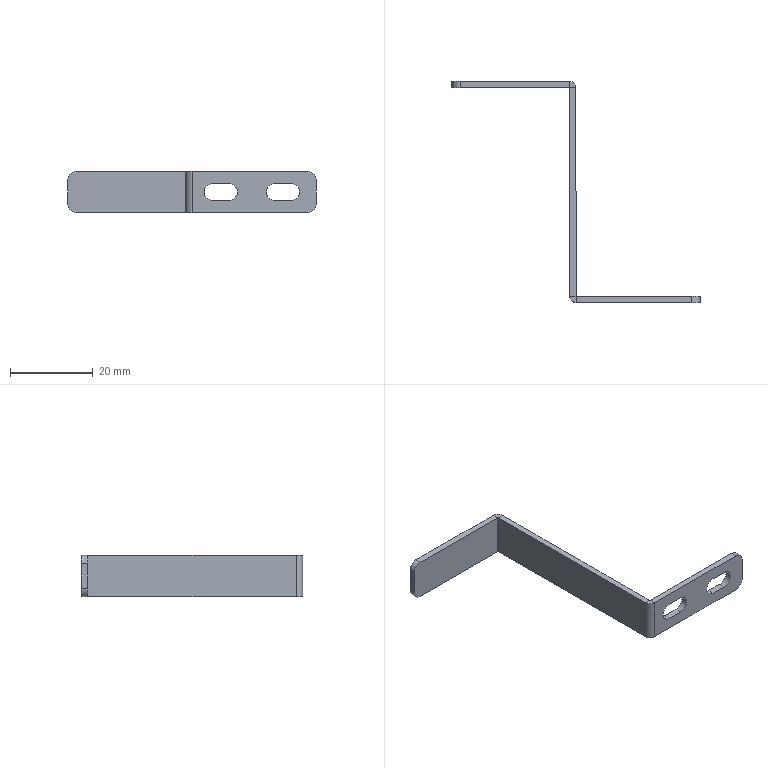Part | SolidWorks | features BreakCorner 1, FlatPattern 1, HoleWzd 1, SMBaseFlange 1, SheetMetal 1 | 1 solid | 34 faces | box 60 x 53.5 x 10 mm | volume 1574 mm3 | plane 22 | cylinder 12 | commonest cylinder face diameters 4 x4 4.2 x4 0.2 x2 3.2 x2
STEP:
#1=CARTESIAN_POINT('',(30.,-1.6,5.));
#2=VERTEX_POINT('',#1);
#3=CARTESIAN_POINT('',(28.5,-1.6,5.));
#4=VERTEX_POINT('',#3);
#5=CARTESIAN_POINT('',(30.,-1.6,5.));
#6=DIRECTION('',(-1.,0.,0.));
#7=VECTOR('',#6,1000.);
#8=LINE('',#5,#7);
#9=EDGE_CURVE('',#2,#4,#8,.T.);
#10=ORIENTED_EDGE('',*,*,#9,.F.);
#11=CARTESIAN_POINT('',(28.4,0.,5.));
#12=VERTEX_POINT('',#11);
#13=CARTESIAN_POINT('',(28.4,-1.6,5.));
#14=DIRECTION('',(0.,0.,-1.));
#15=DIRECTION('',(1.,0.,0.));
#16=AXIS2_PLACEMENT_3D('',#13,#14,#15);
#17=CIRCLE('',#16,1.6);
#18=EDGE_CURVE('',#12,#2,#17,.T.);
#19=ORIENTED_EDGE('',*,*,#18,.F.);
#20=CARTESIAN_POINT('',(28.4,-1.5,5.));
#21=VERTEX_POINT('',#20);
#22=CARTESIAN_POINT('',(28.4,-1.5,5.));
#23=DIRECTION('',(0.,1.,0.));
#24=VECTOR('',#23,1000.);
#25=LINE('',#22,#24);
#26=EDGE_CURVE('',#21,#12,#25,.T.);
#27=ORIENTED_EDGE('',*,*,#26,.F.);
#28=CARTESIAN_POINT('',(28.4,-1.6,5.));
#29=DIRECTION('',(0.,0.,-1.));
#30=DIRECTION('',(1.,0.,0.));
#31=AXIS2_PLACEMENT_3D('',#28,#29,#30);
#32=CIRCLE('',#31,0.1);
#33=EDGE_CURVE('',#21,#4,#32,.T.);
#34=ORIENTED_EDGE('',*,*,#33,.T.);
#35=EDGE_LOOP('',(#10,#19,#27,#34));
#36=FACE_OUTER_BOUND('',#35,.T.);
#37=CARTESIAN_POINT('',(30.,-1.6,5.));
#38=DIRECTION('',(0.,0.,1.));
#39=DIRECTION('',(1.,0.,0.));
#40=AXIS2_PLACEMENT_3D('',#37,#38,#39);
#41=PLANE('',#40);
#42=ADVANCED_FACE('',(#36),#41,.T.);
#43=CARTESIAN_POINT('',(30.,-51.9,5.));
#44=VERTEX_POINT('',#43);
#45=CARTESIAN_POINT('',(30.,0.,5.));
#46=DIRECTION('',(0.,-1.,0.));
#47=VECTOR('',#46,1000.);
#48=LINE('',#45,#47);
#49=EDGE_CURVE('',#2,#44,#48,.T.);
#50=ORIENTED_EDGE('',*,*,#49,.F.);
#51=ORIENTED_EDGE('',*,*,#9,.T.);
#52=CARTESIAN_POINT('',(28.5,-51.9,5.));
#53=VERTEX_POINT('',#52);
#54=CARTESIAN_POINT('',(28.5,0.,5.));
#55=DIRECTION('',(0.,-1.,0.));
#56=VECTOR('',#55,1000.);
#57=LINE('',#54,#56);
#58=EDGE_CURVE('',#4,#53,#57,.T.);
#59=ORIENTED_EDGE('',*,*,#58,.T.);
#60=CARTESIAN_POINT('',(28.5,-51.9,5.));
#61=DIRECTION('',(1.,0.,0.));
#62=VECTOR('',#61,1000.);
#63=LINE('',#60,#62);
#64=EDGE_CURVE('',#53,#44,#63,.T.);
#65=ORIENTED_EDGE('',*,*,#64,.T.);
#66=EDGE_LOOP('',(#50,#51,#59,#65));
#67=FACE_OUTER_BOUND('',#66,.T.);
#68=CARTESIAN_POINT('',(28.4,-1.5,5.));
#69=DIRECTION('',(0.,0.,1.));
#70=DIRECTION('',(1.,0.,0.));
#71=AXIS2_PLACEMENT_3D('',#68,#69,#70);
#72=PLANE('',#71);
#73=ADVANCED_FACE('',(#67),#72,.T.);
#74=CARTESIAN_POINT('',(28.4,0.,-5.));
#75=VERTEX_POINT('',#74);
#76=CARTESIAN_POINT('',(28.4,-1.5,-5.));
#77=VERTEX_POINT('',#76);
#78=CARTESIAN_POINT('',(28.4,0.,-5.));
#79=DIRECTION('',(0.,-1.,0.));
#80=VECTOR('',#79,1000.);
#81=LINE('',#78,#80);
#82=EDGE_CURVE('',#75,#77,#81,.T.);
#83=ORIENTED_EDGE('',*,*,#82,.F.);
#84=CARTESIAN_POINT('',(30.,-1.6,-5.));
#85=VERTEX_POINT('',#84);
#86=CARTESIAN_POINT('',(28.4,-1.6,-5.));
#87=DIRECTION('',(0.,0.,-1.));
#88=DIRECTION('',(1.,0.,0.));
#89=AXIS2_PLACEMENT_3D('',#86,#87,#88);
#90=CIRCLE('',#89,1.6);
#91=EDGE_CURVE('',#75,#85,#90,.T.);
#92=ORIENTED_EDGE('',*,*,#91,.T.);
#93=CARTESIAN_POINT('',(28.5,-1.6,-5.));
#94=VERTEX_POINT('',#93);
#95=CARTESIAN_POINT('',(28.5,-1.6,-5.));
#96=DIRECTION('',(1.,0.,0.));
#97=VECTOR('',#96,1000.);
#98=LINE('',#95,#97);
#99=EDGE_CURVE('',#94,#85,#98,.T.);
#100=ORIENTED_EDGE('',*,*,#99,.F.);
#101=CARTESIAN_POINT('',(28.4,-1.6,-5.));
#102=DIRECTION('',(0.,0.,-1.));
#103=DIRECTION('',(1.,0.,0.));
#104=AXIS2_PLACEMENT_3D('',#101,#102,#103);
#105=CIRCLE('',#104,0.1);
#106=EDGE_CURVE('',#77,#94,#105,.T.);
#107=ORIENTED_EDGE('',*,*,#106,.F.);
#108=EDGE_LOOP('',(#83,#92,#100,#107));
#109=FACE_OUTER_BOUND('',#108,.T.);
#110=CARTESIAN_POINT('',(28.4,0.,-5.));
#111=DIRECTION('',(0.,0.,-1.));
#112=DIRECTION('',(-1.,0.,0.));
#113=AXIS2_PLACEMENT_3D('',#110,#111,#112);
#114=PLANE('',#113);
#115=ADVANCED_FACE('',(#109),#114,.T.);
#116=CARTESIAN_POINT('',(2.,-1.5,-5.));
#117=VERTEX_POINT('',#116);
#118=CARTESIAN_POINT('',(0.,-1.5,-5.));
#119=DIRECTION('',(1.,0.,0.));
#120=VECTOR('',#119,1000.);
#121=LINE('',#118,#120);
#122=EDGE_CURVE('',#117,#77,#121,.T.);
#123=ORIENTED_EDGE('',*,*,#122,.F.);
#124=CARTESIAN_POINT('',(2.,0.,-5.));
#125=VERTEX_POINT('',#124);
#126=CARTESIAN_POINT('',(2.,-1.6,-5.));
#127=DIRECTION('',(0.,1.,0.));
#128=VECTOR('',#127,1000.);
#129=LINE('',#126,#128);
#130=EDGE_CURVE('',#117,#125,#129,.T.);
#131=ORIENTED_EDGE('',*,*,#130,.T.);
#132=CARTESIAN_POINT('',(0.,0.,-5.));
#133=DIRECTION('',(1.,0.,0.));
#134=VECTOR('',#133,1000.);
#135=LINE('',#132,#134);
#136=EDGE_CURVE('',#125,#75,#135,.T.);
#137=ORIENTED_EDGE('',*,*,#136,.T.);
#138=ORIENTED_EDGE('',*,*,#82,.T.);
#139=EDGE_LOOP('',(#123,#131,#137,#138));
#140=FACE_OUTER_BOUND('',#139,.T.);
#141=CARTESIAN_POINT('',(28.5,-1.6,-5.));
#142=DIRECTION('',(0.,0.,-1.));
#143=DIRECTION('',(-1.,0.,0.));
#144=AXIS2_PLACEMENT_3D('',#141,#142,#143);
#145=PLANE('',#144);
#146=ADVANCED_FACE('',(#140),#145,.T.);
#147=CARTESIAN_POINT('',(30.1,-52.,5.));
#148=VERTEX_POINT('',#147);
#149=CARTESIAN_POINT('',(30.1,-53.5,5.));
#150=VERTEX_POINT('',#149);
#151=CARTESIAN_POINT('',(30.1,-52.,5.));
#152=DIRECTION('',(0.,-1.,0.));
#153=VECTOR('',#152,1000.);
#154=LINE('',#151,#153);
#155=EDGE_CURVE('',#148,#150,#154,.T.);
#156=ORIENTED_EDGE('',*,*,#155,.F.);
#157=CARTESIAN_POINT('',(30.1,-51.9,5.));
#158=DIRECTION('',(0.,0.,1.));
#159=DIRECTION('',(-1.,0.,0.));
#160=AXIS2_PLACEMENT_3D('',#157,#158,#159);
#161=CIRCLE('',#160,0.1);
#162=EDGE_CURVE('',#44,#148,#161,.T.);
#163=ORIENTED_EDGE('',*,*,#162,.F.);
#164=ORIENTED_EDGE('',*,*,#64,.F.);
#165=CARTESIAN_POINT('',(30.1,-51.9,5.));
#166=DIRECTION('',(0.,0.,1.));
#167=DIRECTION('',(1.,0.,0.));
#168=AXIS2_PLACEMENT_3D('',#165,#166,#167);
#169=CIRCLE('',#168,1.6);
#170=EDGE_CURVE('',#53,#150,#169,.T.);
#171=ORIENTED_EDGE('',*,*,#170,.T.);
#172=EDGE_LOOP('',(#156,#163,#164,#171));
#173=FACE_OUTER_BOUND('',#172,.T.);
#174=CARTESIAN_POINT('',(30.1,-52.,5.));
#175=DIRECTION('',(0.,0.,1.));
#176=DIRECTION('',(1.,0.,0.));
#177=AXIS2_PLACEMENT_3D('',#174,#175,#176);
#178=PLANE('',#177);
#179=ADVANCED_FACE('',(#173),#178,.T.);
#180=CARTESIAN_POINT('',(58.,-53.5,5.));
#181=VERTEX_POINT('',#180);
#182=CARTESIAN_POINT('',(30.,-53.5,5.));
#183=DIRECTION('',(1.,0.,0.));
#184=VECTOR('',#183,1000.);
#185=LINE('',#182,#184);
#186=EDGE_CURVE('',#150,#181,#185,.T.);
#187=ORIENTED_EDGE('',*,*,#186,.T.);
#188=CARTESIAN_POINT('',(58.,-52.,5.));
#189=VERTEX_POINT('',#188);
#190=CARTESIAN_POINT('',(58.,-51.9,5.));
#191=DIRECTION('',(0.,1.,0.));
#192=VECTOR('',#191,1000.);
#193=LINE('',#190,#192);
#194=EDGE_CURVE('',#181,#189,#193,.T.);
#195=ORIENTED_EDGE('',*,*,#194,.T.);
#196=CARTESIAN_POINT('',(30.,-52.,5.));
#197=DIRECTION('',(1.,0.,0.));
#198=VECTOR('',#197,1000.);
#199=LINE('',#196,#198);
#200=EDGE_CURVE('',#148,#189,#199,.T.);
#201=ORIENTED_EDGE('',*,*,#200,.F.);
#202=ORIENTED_EDGE('',*,*,#155,.T.);
#203=EDGE_LOOP('',(#187,#195,#201,#202));
#204=FACE_OUTER_BOUND('',#203,.T.);
#205=CARTESIAN_POINT('',(28.5,-51.9,5.));
#206=DIRECTION('',(0.,0.,1.));
#207=DIRECTION('',(1.,0.,0.));
#208=AXIS2_PLACEMENT_3D('',#205,#206,#207);
#209=PLANE('',#208);
#210=ADVANCED_FACE('',(#204),#209,.T.);
#211=CARTESIAN_POINT('',(30.,-51.9,-5.));
#212=VERTEX_POINT('',#211);
#213=CARTESIAN_POINT('',(28.5,-51.9,-5.));
#214=VERTEX_POINT('',#213);
#215=CARTESIAN_POINT('',(30.,-51.9,-5.));
#216=DIRECTION('',(-1.,0.,0.));
#217=VECTOR('',#216,1000.);
#218=LINE('',#215,#217);
#219=EDGE_CURVE('',#212,#214,#218,.T.);
#220=ORIENTED_EDGE('',*,*,#219,.F.);
#221=CARTESIAN_POINT('',(30.1,-52.,-5.));
#222=VERTEX_POINT('',#221);
#223=CARTESIAN_POINT('',(30.1,-51.9,-5.));
#224=DIRECTION('',(0.,0.,1.));
#225=DIRECTION('',(-1.,0.,0.));
#226=AXIS2_PLACEMENT_3D('',#223,#224,#225);
#227=CIRCLE('',#226,0.1);
#228=EDGE_CURVE('',#212,#222,#227,.T.);
#229=ORIENTED_EDGE('',*,*,#228,.T.);
#230=CARTESIAN_POINT('',(30.1,-53.5,-5.));
#231=VERTEX_POINT('',#230);
#232=CARTESIAN_POINT('',(30.1,-53.5,-5.));
#233=DIRECTION('',(0.,1.,0.));
#234=VECTOR('',#233,1000.);
#235=LINE('',#232,#234);
#236=EDGE_CURVE('',#231,#222,#235,.T.);
#237=ORIENTED_EDGE('',*,*,#236,.F.);
#238=CARTESIAN_POINT('',(30.1,-51.9,-5.));
#239=DIRECTION('',(0.,0.,1.));
#240=DIRECTION('',(1.,0.,0.));
#241=AXIS2_PLACEMENT_3D('',#238,#239,#240);
#242=CIRCLE('',#241,1.6);
#243=EDGE_CURVE('',#214,#231,#242,.T.);
#244=ORIENTED_EDGE('',*,*,#243,.F.);
#245=EDGE_LOOP('',(#220,#229,#237,#244));
#246=FACE_OUTER_BOUND('',#245,.T.);
#247=CARTESIAN_POINT('',(30.,-51.9,-5.));
#248=DIRECTION('',(0.,0.,-1.));
#249=DIRECTION('',(-1.,0.,0.));
#250=AXIS2_PLACEMENT_3D('',#247,#248,#249);
#251=PLANE('',#250);
#252=ADVANCED_FACE('',(#246),#251,.T.);
#253=CARTESIAN_POINT('',(30.,0.,-5.));
#254=DIRECTION('',(0.,-1.,0.));
#255=VECTOR('',#254,1000.);
#256=LINE('',#253,#255);
#257=EDGE_CURVE('',#85,#212,#256,.T.);
#258=ORIENTED_EDGE('',*,*,#257,.T.);
#259=ORIENTED_EDGE('',*,*,#219,.T.);
#260=CARTESIAN_POINT('',(28.5,0.,-5.));
#261=DIRECTION('',(0.,-1.,0.));
#262=VECTOR('',#261,1000.);
#263=LINE('',#260,#262);
#264=EDGE_CURVE('',#94,#214,#263,.T.);
#265=ORIENTED_EDGE('',*,*,#264,.F.);
#266=ORIENTED_EDGE('',*,*,#99,.T.);
#267=EDGE_LOOP('',(#258,#259,#265,#266));
#268=FACE_OUTER_BOUND('',#267,.T.);
#269=CARTESIAN_POINT('',(30.1,-53.5,-5.));
#270=DIRECTION('',(0.,0.,-1.));
#271=DIRECTION('',(-1.,0.,0.));
#272=AXIS2_PLACEMENT_3D('',#269,#270,#271);
#273=PLANE('',#272);
#274=ADVANCED_FACE('',(#268),#273,.T.);
#275=CARTESIAN_POINT('',(38.9,-53.5,2.1));
#276=VERTEX_POINT('',#275);
#277=CARTESIAN_POINT('',(38.9,-53.5,-2.1));
#278=VERTEX_POINT('',#277);
#279=CARTESIAN_POINT('',(38.9,-53.5,0.));
#280=DIRECTION('',(0.,1.,0.));
#281=DIRECTION('',(-1.,0.,0.));
#282=AXIS2_PLACEMENT_3D('',#279,#280,#281);
#283=CIRCLE('',#282,2.1);
#284=EDGE_CURVE('',#276,#278,#283,.T.);
#285=ORIENTED_EDGE('',*,*,#284,.T.);
#286=CARTESIAN_POINT('',(35.1,-53.5,-2.1));
#287=VERTEX_POINT('',#286);
#288=CARTESIAN_POINT('',(30.,-53.5,-2.1));
#289=DIRECTION('',(-1.,0.,0.));
#290=VECTOR('',#289,1000.);
#291=LINE('',#288,#290);
#292=EDGE_CURVE('',#278,#287,#291,.T.);
#293=ORIENTED_EDGE('',*,*,#292,.T.);
#294=CARTESIAN_POINT('',(35.1,-53.5,2.1));
#295=VERTEX_POINT('',#294);
#296=CARTESIAN_POINT('',(35.1,-53.5,0.));
#297=DIRECTION('',(0.,1.,0.));
#298=DIRECTION('',(-1.,0.,0.));
#299=AXIS2_PLACEMENT_3D('',#296,#297,#298);
#300=CIRCLE('',#299,2.1);
#301=EDGE_CURVE('',#287,#295,#300,.T.);
#302=ORIENTED_EDGE('',*,*,#301,.T.);
#303=CARTESIAN_POINT('',(30.,-53.5,2.1));
#304=DIRECTION('',(1.,0.,0.));
#305=VECTOR('',#304,1000.);
#306=LINE('',#303,#305);
#307=EDGE_CURVE('',#295,#276,#306,.T.);
#308=ORIENTED_EDGE('',*,*,#307,.T.);
#309=EDGE_LOOP('',(#285,#293,#302,#308));
#310=FACE_BOUND('',#309,.T.);
#311=CARTESIAN_POINT('',(53.9,-53.5,2.1));
#312=VERTEX_POINT('',#311);
#313=CARTESIAN_POINT('',(53.9,-53.5,-2.1));
#314=VERTEX_POINT('',#313);
#315=CARTESIAN_POINT('',(53.9,-53.5,0.));
#316=DIRECTION('',(0.,1.,0.));
#317=DIRECTION('',(-1.,0.,0.));
#318=AXIS2_PLACEMENT_3D('',#315,#316,#317);
#319=CIRCLE('',#318,2.1);
#320=EDGE_CURVE('',#312,#314,#319,.T.);
#321=ORIENTED_EDGE('',*,*,#320,.T.);
#322=CARTESIAN_POINT('',(50.1,-53.5,-2.1));
#323=VERTEX_POINT('',#322);
#324=CARTESIAN_POINT('',(30.,-53.5,-2.1));
#325=DIRECTION('',(-1.,0.,0.));
#326=VECTOR('',#325,1000.);
#327=LINE('',#324,#326);
#328=EDGE_CURVE('',#314,#323,#327,.T.);
#329=ORIENTED_EDGE('',*,*,#328,.T.);
#330=CARTESIAN_POINT('',(50.1,-53.5,2.1));
#331=VERTEX_POINT('',#330);
#332=CARTESIAN_POINT('',(50.1,-53.5,0.));
#333=DIRECTION('',(0.,1.,0.));
#334=DIRECTION('',(-1.,0.,0.));
#335=AXIS2_PLACEMENT_3D('',#332,#333,#334);
#336=CIRCLE('',#335,2.1);
#337=EDGE_CURVE('',#323,#331,#336,.T.);
#338=ORIENTED_EDGE('',*,*,#337,.T.);
#339=CARTESIAN_POINT('',(30.,-53.5,2.1));
#340=DIRECTION('',(1.,0.,0.));
#341=VECTOR('',#340,1000.);
#342=LINE('',#339,#341);
#343=EDGE_CURVE('',#331,#312,#342,.T.);
#344=ORIENTED_EDGE('',*,*,#343,.T.);
#345=EDGE_LOOP('',(#321,#329,#338,#344));
#346=FACE_BOUND('',#345,.T.);
#347=CARTESIAN_POINT('',(60.,-53.5,3.));
#348=VERTEX_POINT('',#347);
#349=CARTESIAN_POINT('',(60.,-53.5,-3.));
#350=VERTEX_POINT('',#349);
#351=CARTESIAN_POINT('',(60.,-53.5,5.));
#352=DIRECTION('',(0.,0.,-1.));
#353=VECTOR('',#352,1000.);
#354=LINE('',#351,#353);
#355=EDGE_CURVE('',#348,#350,#354,.T.);
#356=ORIENTED_EDGE('',*,*,#355,.F.);
#357=CARTESIAN_POINT('',(58.,-53.5,3.));
#358=DIRECTION('',(0.,-1.,0.));
#359=DIRECTION('',(-1.,0.,0.));
#360=AXIS2_PLACEMENT_3D('',#357,#358,#359);
#361=CIRCLE('',#360,2.);
#362=EDGE_CURVE('',#348,#181,#361,.T.);
#363=ORIENTED_EDGE('',*,*,#362,.T.);
#364=ORIENTED_EDGE('',*,*,#186,.F.);
#365=CARTESIAN_POINT('',(30.1,-53.5,5.));
#366=DIRECTION('',(0.,0.,-1.));
#367=VECTOR('',#366,1000.);
#368=LINE('',#365,#367);
#369=EDGE_CURVE('',#150,#231,#368,.T.);
#370=ORIENTED_EDGE('',*,*,#369,.T.);
#371=CARTESIAN_POINT('',(58.,-53.5,-5.));
#372=VERTEX_POINT('',#371);
#373=CARTESIAN_POINT('',(30.,-53.5,-5.));
#374=DIRECTION('',(1.,0.,0.));
#375=VECTOR('',#374,1000.);
#376=LINE('',#373,#375);
#377=EDGE_CURVE('',#231,#372,#376,.T.);
#378=ORIENTED_EDGE('',*,*,#377,.T.);
#379=CARTESIAN_POINT('',(58.,-53.5,-3.));
#380=DIRECTION('',(0.,-1.,0.));
#381=DIRECTION('',(-1.,0.,0.));
#382=AXIS2_PLACEMENT_3D('',#379,#380,#381);
#383=CIRCLE('',#382,2.);
#384=EDGE_CURVE('',#372,#350,#383,.T.);
#385=ORIENTED_EDGE('',*,*,#384,.T.);
#386=EDGE_LOOP('',(#356,#363,#364,#370,#378,#385));
#387=FACE_OUTER_BOUND('',#386,.T.);
#388=CARTESIAN_POINT('',(30.,-53.5,5.));
#389=DIRECTION('',(0.,1.,0.));
#390=DIRECTION('',(-1.,0.,0.));
#391=AXIS2_PLACEMENT_3D('',#388,#389,#390);
#392=PLANE('',#391);
#393=ADVANCED_FACE('',(#310,#346,#387),#392,.F.);
#394=CARTESIAN_POINT('',(60.,-52.,3.));
#395=VERTEX_POINT('',#394);
#396=CARTESIAN_POINT('',(60.,-52.,-3.));
#397=VERTEX_POINT('',#396);
#398=CARTESIAN_POINT('',(60.,-52.,5.));
#399=DIRECTION('',(0.,0.,-1.));
#400=VECTOR('',#399,1000.);
#401=LINE('',#398,#400);
#402=EDGE_CURVE('',#395,#397,#401,.T.);
#403=ORIENTED_EDGE('',*,*,#402,.F.);
#404=CARTESIAN_POINT('',(60.,-52.,3.));
#405=DIRECTION('',(0.,-1.,0.));
#406=VECTOR('',#405,1000.);
#407=LINE('',#404,#406);
#408=EDGE_CURVE('',#395,#348,#407,.T.);
#409=ORIENTED_EDGE('',*,*,#408,.T.);
#410=ORIENTED_EDGE('',*,*,#355,.T.);
#411=CARTESIAN_POINT('',(60.,-52.,-3.));
#412=DIRECTION('',(0.,1.,0.));
#413=VECTOR('',#412,1000.);
#414=LINE('',#411,#413);
#415=EDGE_CURVE('',#350,#397,#414,.T.);
#416=ORIENTED_EDGE('',*,*,#415,.T.);
#417=EDGE_LOOP('',(#403,#409,#410,#416));
#418=FACE_OUTER_BOUND('',#417,.T.);
#419=CARTESIAN_POINT('',(60.,-52.,5.));
#420=DIRECTION('',(1.,0.,0.));
#421=DIRECTION('',(0.,0.,-1.));
#422=AXIS2_PLACEMENT_3D('',#419,#420,#421);
#423=PLANE('',#422);
#424=ADVANCED_FACE('',(#418),#423,.T.);
#425=CARTESIAN_POINT('',(38.9,-52.,2.1));
#426=VERTEX_POINT('',#425);
#427=CARTESIAN_POINT('',(38.9,-52.,-2.1));
#428=VERTEX_POINT('',#427);
#429=CARTESIAN_POINT('',(38.9,-52.,0.));
#430=DIRECTION('',(0.,1.,0.));
#431=DIRECTION('',(0.,0.,1.));
#432=AXIS2_PLACEMENT_3D('',#429,#430,#431);
#433=CIRCLE('',#432,2.1);
#434=EDGE_CURVE('',#426,#428,#433,.T.);
#435=ORIENTED_EDGE('',*,*,#434,.F.);
#436=CARTESIAN_POINT('',(35.1,-52.,2.1));
#437=VERTEX_POINT('',#436);
#438=CARTESIAN_POINT('',(35.1,-52.,2.1));
#439=DIRECTION('',(1.,0.,0.));
#440=VECTOR('',#439,1000.);
#441=LINE('',#438,#440);
#442=EDGE_CURVE('',#437,#426,#441,.T.);
#443=ORIENTED_EDGE('',*,*,#442,.F.);
#444=CARTESIAN_POINT('',(35.1,-52.,-2.1));
#445=VERTEX_POINT('',#444);
#446=CARTESIAN_POINT('',(35.1,-52.,0.));
#447=DIRECTION('',(0.,1.,0.));
#448=DIRECTION('',(0.,0.,1.));
#449=AXIS2_PLACEMENT_3D('',#446,#447,#448);
#450=CIRCLE('',#449,2.1);
#451=EDGE_CURVE('',#445,#437,#450,.T.);
#452=ORIENTED_EDGE('',*,*,#451,.F.);
#453=CARTESIAN_POINT('',(35.1,-52.,-2.1));
#454=DIRECTION('',(1.,0.,0.));
#455=VECTOR('',#454,1000.);
#456=LINE('',#453,#455);
#457=EDGE_CURVE('',#445,#428,#456,.T.);
#458=ORIENTED_EDGE('',*,*,#457,.T.);
#459=EDGE_LOOP('',(#435,#443,#452,#458));
#460=FACE_BOUND('',#459,.T.);
#461=CARTESIAN_POINT('',(50.1,-52.,2.1));
#462=VERTEX_POINT('',#461);
#463=CARTESIAN_POINT('',(53.9,-52.,2.1));
#464=VERTEX_POINT('',#463);
#465=CARTESIAN_POINT('',(50.1,-52.,2.1));
#466=DIRECTION('',(1.,0.,0.));
#467=VECTOR('',#466,1000.);
#468=LINE('',#465,#467);
#469=EDGE_CURVE('',#462,#464,#468,.T.);
#470=ORIENTED_EDGE('',*,*,#469,.F.);
#471=CARTESIAN_POINT('',(50.1,-52.,-2.1));
#472=VERTEX_POINT('',#471);
#473=CARTESIAN_POINT('',(50.1,-52.,0.));
#474=DIRECTION('',(0.,1.,0.));
#475=DIRECTION('',(0.,0.,1.));
#476=AXIS2_PLACEMENT_3D('',#473,#474,#475);
#477=CIRCLE('',#476,2.1);
#478=EDGE_CURVE('',#472,#462,#477,.T.);
#479=ORIENTED_EDGE('',*,*,#478,.F.);
#480=CARTESIAN_POINT('',(53.9,-52.,-2.1));
#481=VERTEX_POINT('',#480);
#482=CARTESIAN_POINT('',(50.1,-52.,-2.1));
#483=DIRECTION('',(1.,0.,0.));
#484=VECTOR('',#483,1000.);
#485=LINE('',#482,#484);
#486=EDGE_CURVE('',#472,#481,#485,.T.);
#487=ORIENTED_EDGE('',*,*,#486,.T.);
#488=CARTESIAN_POINT('',(53.9,-52.,0.));
#489=DIRECTION('',(0.,1.,0.));
#490=DIRECTION('',(0.,0.,1.));
#491=AXIS2_PLACEMENT_3D('',#488,#489,#490);
#492=CIRCLE('',#491,2.1);
#493=EDGE_CURVE('',#464,#481,#492,.T.);
#494=ORIENTED_EDGE('',*,*,#493,.F.);
#495=EDGE_LOOP('',(#470,#479,#487,#494));
#496=FACE_BOUND('',#495,.T.);
#497=ORIENTED_EDGE('',*,*,#200,.T.);
#498=CARTESIAN_POINT('',(58.,-52.,3.));
#499=DIRECTION('',(0.,1.,0.));
#500=DIRECTION('',(-1.,0.,0.));
#501=AXIS2_PLACEMENT_3D('',#498,#499,#500);
#502=CIRCLE('',#501,2.);
#503=EDGE_CURVE('',#189,#395,#502,.T.);
#504=ORIENTED_EDGE('',*,*,#503,.T.);
#505=ORIENTED_EDGE('',*,*,#402,.T.);
#506=CARTESIAN_POINT('',(58.,-52.,-5.));
#507=VERTEX_POINT('',#506);
#508=CARTESIAN_POINT('',(58.,-52.,-3.));
#509=DIRECTION('',(0.,1.,0.));
#510=DIRECTION('',(-1.,0.,0.));
#511=AXIS2_PLACEMENT_3D('',#508,#509,#510);
#512=CIRCLE('',#511,2.);
#513=EDGE_CURVE('',#397,#507,#512,.T.);
#514=ORIENTED_EDGE('',*,*,#513,.T.);
#515=CARTESIAN_POINT('',(30.,-52.,-5.));
#516=DIRECTION('',(1.,0.,0.));
#517=VECTOR('',#516,1000.);
#518=LINE('',#515,#517);
#519=EDGE_CURVE('',#222,#507,#518,.T.);
#520=ORIENTED_EDGE('',*,*,#519,.F.);
#521=CARTESIAN_POINT('',(30.1,-52.,5.));
#522=DIRECTION('',(0.,0.,-1.));
#523=VECTOR('',#522,1000.);
#524=LINE('',#521,#523);
#525=EDGE_CURVE('',#148,#222,#524,.T.);
#526=ORIENTED_EDGE('',*,*,#525,.F.);
#527=EDGE_LOOP('',(#497,#504,#505,#514,#520,#526));
#528=FACE_OUTER_BOUND('',#527,.T.);
#529=CARTESIAN_POINT('',(30.,-52.,5.));
#530=DIRECTION('',(0.,1.,0.));
#531=DIRECTION('',(-1.,0.,0.));
#532=AXIS2_PLACEMENT_3D('',#529,#530,#531);
#533=PLANE('',#532);
#534=ADVANCED_FACE('',(#460,#496,#528),#533,.T.);
#535=ORIENTED_EDGE('',*,*,#228,.F.);
#536=CARTESIAN_POINT('',(30.,-51.9,5.));
#537=DIRECTION('',(0.,0.,-1.));
#538=VECTOR('',#537,1000.);
#539=LINE('',#536,#538);
#540=EDGE_CURVE('',#44,#212,#539,.T.);
#541=ORIENTED_EDGE('',*,*,#540,.F.);
#542=ORIENTED_EDGE('',*,*,#162,.T.);
#543=ORIENTED_EDGE('',*,*,#525,.T.);
#544=EDGE_LOOP('',(#535,#541,#542,#543));
#545=FACE_OUTER_BOUND('',#544,.T.);
#546=CARTESIAN_POINT('',(30.1,-51.9,5.));
#547=DIRECTION('',(0.,0.,-1.));
#548=DIRECTION('',(-1.,0.,0.));
#549=AXIS2_PLACEMENT_3D('',#546,#547,#548);
#550=CYLINDRICAL_SURFACE('',#549,0.1);
#551=ADVANCED_FACE('',(#545),#550,.F.);
#552=ORIENTED_EDGE('',*,*,#257,.F.);
#553=CARTESIAN_POINT('',(30.,-1.6,5.));
#554=DIRECTION('',(0.,0.,-1.));
#555=VECTOR('',#554,1000.);
#556=LINE('',#553,#555);
#557=EDGE_CURVE('',#2,#85,#556,.T.);
#558=ORIENTED_EDGE('',*,*,#557,.F.);
#559=ORIENTED_EDGE('',*,*,#49,.T.);
#560=ORIENTED_EDGE('',*,*,#540,.T.);
#561=EDGE_LOOP('',(#552,#558,#559,#560));
#562=FACE_OUTER_BOUND('',#561,.T.);
#563=CARTESIAN_POINT('',(30.,0.,5.));
#564=DIRECTION('',(1.,0.,0.));
#565=DIRECTION('',(0.,1.,0.));
#566=AXIS2_PLACEMENT_3D('',#563,#564,#565);
#567=PLANE('',#566);
#568=ADVANCED_FACE('',(#562),#567,.T.);
#569=ORIENTED_EDGE('',*,*,#91,.F.);
#570=CARTESIAN_POINT('',(28.4,0.,5.));
#571=DIRECTION('',(0.,0.,-1.));
#572=VECTOR('',#571,1000.);
#573=LINE('',#570,#572);
#574=EDGE_CURVE('',#12,#75,#573,.T.);
#575=ORIENTED_EDGE('',*,*,#574,.F.);
#576=ORIENTED_EDGE('',*,*,#18,.T.);
#577=ORIENTED_EDGE('',*,*,#557,.T.);
#578=EDGE_LOOP('',(#569,#575,#576,#577));
#579=FACE_OUTER_BOUND('',#578,.T.);
#580=CARTESIAN_POINT('',(28.4,-1.6,5.));
#581=DIRECTION('',(0.,0.,-1.));
#582=DIRECTION('',(-1.,0.,0.));
#583=AXIS2_PLACEMENT_3D('',#580,#581,#582);
#584=CYLINDRICAL_SURFACE('',#583,1.6);
#585=ADVANCED_FACE('',(#579),#584,.T.);
#586=ORIENTED_EDGE('',*,*,#136,.F.);
#587=CARTESIAN_POINT('',(0.,0.,-3.));
#588=VERTEX_POINT('',#587);
#589=CARTESIAN_POINT('',(2.,0.,-3.));
#590=DIRECTION('',(0.,1.,0.));
#591=DIRECTION('',(0.,0.,1.));
#592=AXIS2_PLACEMENT_3D('',#589,#590,#591);
#593=CIRCLE('',#592,2.);
#594=EDGE_CURVE('',#125,#588,#593,.T.);
#595=ORIENTED_EDGE('',*,*,#594,.T.);
#596=CARTESIAN_POINT('',(0.,0.,3.));
#597=VERTEX_POINT('',#596);
#598=CARTESIAN_POINT('',(0.,0.,5.));
#599=DIRECTION('',(0.,0.,-1.));
#600=VECTOR('',#599,1000.);
#601=LINE('',#598,#600);
#602=EDGE_CURVE('',#597,#588,#601,.T.);
#603=ORIENTED_EDGE('',*,*,#602,.F.);
#604=CARTESIAN_POINT('',(2.,0.,5.));
#605=VERTEX_POINT('',#604);
#606=CARTESIAN_POINT('',(2.,0.,3.));
#607=DIRECTION('',(0.,1.,0.));
#608=DIRECTION('',(0.,0.,1.));
#609=AXIS2_PLACEMENT_3D('',#606,#607,#608);
#610=CIRCLE('',#609,2.);
#611=EDGE_CURVE('',#597,#605,#610,.T.);
#612=ORIENTED_EDGE('',*,*,#611,.T.);
#613=CARTESIAN_POINT('',(0.,0.,5.));
#614=DIRECTION('',(1.,0.,0.));
#615=VECTOR('',#614,1000.);
#616=LINE('',#613,#615);
#617=EDGE_CURVE('',#605,#12,#616,.T.);
#618=ORIENTED_EDGE('',*,*,#617,.T.);
#619=ORIENTED_EDGE('',*,*,#574,.T.);
#620=EDGE_LOOP('',(#586,#595,#603,#612,#618,#619));
#621=FACE_OUTER_BOUND('',#620,.T.);
#622=CARTESIAN_POINT('',(0.,0.,5.));
#623=DIRECTION('',(0.,1.,0.));
#624=DIRECTION('',(0.,0.,1.));
#625=AXIS2_PLACEMENT_3D('',#622,#623,#624);
#626=PLANE('',#625);
#627=ADVANCED_FACE('',(#621),#626,.T.);
#628=ORIENTED_EDGE('',*,*,#602,.T.);
#629=CARTESIAN_POINT('',(0.,-1.5,-3.));
#630=VERTEX_POINT('',#629);
#631=CARTESIAN_POINT('',(0.,-1.5,-3.));
#632=DIRECTION('',(0.,-1.,0.));
#633=VECTOR('',#632,1000.);
#634=LINE('',#631,#633);
#635=EDGE_CURVE('',#588,#630,#634,.T.);
#636=ORIENTED_EDGE('',*,*,#635,.T.);
#637=CARTESIAN_POINT('',(0.,-1.5,3.));
#638=VERTEX_POINT('',#637);
#639=CARTESIAN_POINT('',(0.,-1.5,5.));
#640=DIRECTION('',(0.,0.,-1.));
#641=VECTOR('',#640,1000.);
#642=LINE('',#639,#641);
#643=EDGE_CURVE('',#638,#630,#642,.T.);
#644=ORIENTED_EDGE('',*,*,#643,.F.);
#645=CARTESIAN_POINT('',(0.,0.,3.));
#646=DIRECTION('',(0.,1.,0.));
#647=VECTOR('',#646,1000.);
#648=LINE('',#645,#647);
#649=EDGE_CURVE('',#638,#597,#648,.T.);
#650=ORIENTED_EDGE('',*,*,#649,.T.);
#651=EDGE_LOOP('',(#628,#636,#644,#650));
#652=FACE_OUTER_BOUND('',#651,.T.);
#653=CARTESIAN_POINT('',(0.,-1.5,5.));
#654=DIRECTION('',(-1.,0.,0.));
#655=DIRECTION('',(0.,0.,1.));
#656=AXIS2_PLACEMENT_3D('',#653,#654,#655);
#657=PLANE('',#656);
#658=ADVANCED_FACE('',(#652),#657,.T.);
#659=ORIENTED_EDGE('',*,*,#643,.T.);
#660=CARTESIAN_POINT('',(2.,-1.5,-3.));
#661=DIRECTION('',(0.,-1.,0.));
#662=DIRECTION('',(0.,0.,1.));
#663=AXIS2_PLACEMENT_3D('',#660,#661,#662);
#664=CIRCLE('',#663,2.);
#665=EDGE_CURVE('',#630,#117,#664,.T.);
#666=ORIENTED_EDGE('',*,*,#665,.T.);
#667=ORIENTED_EDGE('',*,*,#122,.T.);
#668=CARTESIAN_POINT('',(28.4,-1.5,5.));
#669=DIRECTION('',(0.,0.,-1.));
#670=VECTOR('',#669,1000.);
#671=LINE('',#668,#670);
#672=EDGE_CURVE('',#21,#77,#671,.T.);
#673=ORIENTED_EDGE('',*,*,#672,.F.);
#674=CARTESIAN_POINT('',(2.,-1.5,5.));
#675=VERTEX_POINT('',#674);
#676=CARTESIAN_POINT('',(0.,-1.5,5.));
#677=DIRECTION('',(1.,0.,0.));
#678=VECTOR('',#677,1000.);
#679=LINE('',#676,#678);
#680=EDGE_CURVE('',#675,#21,#679,.T.);
#681=ORIENTED_EDGE('',*,*,#680,.F.);
#682=CARTESIAN_POINT('',(2.,-1.5,3.));
#683=DIRECTION('',(0.,-1.,0.));
#684=DIRECTION('',(0.,0.,1.));
#685=AXIS2_PLACEMENT_3D('',#682,#683,#684);
#686=CIRCLE('',#685,2.);
#687=EDGE_CURVE('',#675,#638,#686,.T.);
#688=ORIENTED_EDGE('',*,*,#687,.T.);
#689=EDGE_LOOP('',(#659,#666,#667,#673,#681,#688));
#690=FACE_OUTER_BOUND('',#689,.T.);
#691=CARTESIAN_POINT('',(0.,-1.5,5.));
#692=DIRECTION('',(0.,1.,0.));
#693=DIRECTION('',(0.,0.,1.));
#694=AXIS2_PLACEMENT_3D('',#691,#692,#693);
#695=PLANE('',#694);
#696=ADVANCED_FACE('',(#690),#695,.F.);
#697=ORIENTED_EDGE('',*,*,#106,.T.);
#698=CARTESIAN_POINT('',(28.5,-1.6,5.));
#699=DIRECTION('',(0.,0.,-1.));
#700=VECTOR('',#699,1000.);
#701=LINE('',#698,#700);
#702=EDGE_CURVE('',#4,#94,#701,.T.);
#703=ORIENTED_EDGE('',*,*,#702,.F.);
#704=ORIENTED_EDGE('',*,*,#33,.F.);
#705=ORIENTED_EDGE('',*,*,#672,.T.);
#706=EDGE_LOOP('',(#697,#703,#704,#705));
#707=FACE_OUTER_BOUND('',#706,.T.);
#708=CARTESIAN_POINT('',(28.4,-1.6,5.));
#709=DIRECTION('',(0.,0.,-1.));
#710=DIRECTION('',(-1.,0.,0.));
#711=AXIS2_PLACEMENT_3D('',#708,#709,#710);
#712=CYLINDRICAL_SURFACE('',#711,0.1);
#713=ADVANCED_FACE('',(#707),#712,.F.);
#714=ORIENTED_EDGE('',*,*,#264,.T.);
#715=CARTESIAN_POINT('',(28.5,-51.9,5.));
#716=DIRECTION('',(0.,0.,-1.));
#717=VECTOR('',#716,1000.);
#718=LINE('',#715,#717);
#719=EDGE_CURVE('',#53,#214,#718,.T.);
#720=ORIENTED_EDGE('',*,*,#719,.F.);
#721=ORIENTED_EDGE('',*,*,#58,.F.);
#722=ORIENTED_EDGE('',*,*,#702,.T.);
#723=EDGE_LOOP('',(#714,#720,#721,#722));
#724=FACE_OUTER_BOUND('',#723,.T.);
#725=CARTESIAN_POINT('',(28.5,0.,5.));
#726=DIRECTION('',(1.,0.,0.));
#727=DIRECTION('',(0.,1.,0.));
#728=AXIS2_PLACEMENT_3D('',#725,#726,#727);
#729=PLANE('',#728);
#730=ADVANCED_FACE('',(#724),#729,.F.);
#731=ORIENTED_EDGE('',*,*,#243,.T.);
#732=ORIENTED_EDGE('',*,*,#369,.F.);
#733=ORIENTED_EDGE('',*,*,#170,.F.);
#734=ORIENTED_EDGE('',*,*,#719,.T.);
#735=EDGE_LOOP('',(#731,#732,#733,#734));
#736=FACE_OUTER_BOUND('',#735,.T.);
#737=CARTESIAN_POINT('',(30.1,-51.9,5.));
#738=DIRECTION('',(0.,0.,-1.));
#739=DIRECTION('',(-1.,0.,0.));
#740=AXIS2_PLACEMENT_3D('',#737,#738,#739);
#741=CYLINDRICAL_SURFACE('',#740,1.6);
#742=ADVANCED_FACE('',(#736),#741,.T.);
#743=ORIENTED_EDGE('',*,*,#617,.F.);
#744=CARTESIAN_POINT('',(2.,-1.5,5.));
#745=DIRECTION('',(0.,-1.,0.));
#746=VECTOR('',#745,1000.);
#747=LINE('',#744,#746);
#748=EDGE_CURVE('',#605,#675,#747,.T.);
#749=ORIENTED_EDGE('',*,*,#748,.T.);
#750=ORIENTED_EDGE('',*,*,#680,.T.);
#751=ORIENTED_EDGE('',*,*,#26,.T.);
#752=EDGE_LOOP('',(#743,#749,#750,#751));
#753=FACE_OUTER_BOUND('',#752,.T.);
#754=CARTESIAN_POINT('',(30.1,-51.9,5.));
#755=DIRECTION('',(0.,0.,-1.));
#756=DIRECTION('',(-1.,0.,0.));
#757=AXIS2_PLACEMENT_3D('',#754,#755,#756);
#758=PLANE('',#757);
#759=ADVANCED_FACE('',(#753),#758,.F.);
#760=ORIENTED_EDGE('',*,*,#519,.T.);
#761=CARTESIAN_POINT('',(58.,-51.9,-5.));
#762=DIRECTION('',(0.,-1.,0.));
#763=VECTOR('',#762,1000.);
#764=LINE('',#761,#763);
#765=EDGE_CURVE('',#507,#372,#764,.T.);
#766=ORIENTED_EDGE('',*,*,#765,.T.);
#767=ORIENTED_EDGE('',*,*,#377,.F.);
#768=ORIENTED_EDGE('',*,*,#236,.T.);
#769=EDGE_LOOP('',(#760,#766,#767,#768));
#770=FACE_OUTER_BOUND('',#769,.T.);
#771=CARTESIAN_POINT('',(30.1,-51.9,-5.));
#772=DIRECTION('',(0.,0.,-1.));
#773=DIRECTION('',(-1.,0.,0.));
#774=AXIS2_PLACEMENT_3D('',#771,#772,#773);
#775=PLANE('',#774);
#776=ADVANCED_FACE('',(#770),#775,.T.);
#777=CARTESIAN_POINT('',(53.9,-52.,2.1));
#778=DIRECTION('',(0.,-1.,0.));
#779=VECTOR('',#778,1000.);
#780=LINE('',#777,#779);
#781=EDGE_CURVE('',#464,#312,#780,.T.);
#782=ORIENTED_EDGE('',*,*,#781,.F.);
#783=ORIENTED_EDGE('',*,*,#493,.T.);
#784=CARTESIAN_POINT('',(53.9,-52.,-2.1));
#785=DIRECTION('',(0.,1.,0.));
#786=VECTOR('',#785,1000.);
#787=LINE('',#784,#786);
#788=EDGE_CURVE('',#314,#481,#787,.T.);
#789=ORIENTED_EDGE('',*,*,#788,.F.);
#790=ORIENTED_EDGE('',*,*,#320,.F.);
#791=EDGE_LOOP('',(#782,#783,#789,#790));
#792=FACE_OUTER_BOUND('',#791,.T.);
#793=CARTESIAN_POINT('',(53.9,-52.,0.));
#794=DIRECTION('',(0.,1.,0.));
#795=DIRECTION('',(0.,0.,1.));
#796=AXIS2_PLACEMENT_3D('',#793,#794,#795);
#797=CYLINDRICAL_SURFACE('',#796,2.1);
#798=ADVANCED_FACE('',(#792),#797,.F.);
#799=CARTESIAN_POINT('',(50.1,-52.,-2.1));
#800=DIRECTION('',(0.,-1.,0.));
#801=VECTOR('',#800,1000.);
#802=LINE('',#799,#801);
#803=EDGE_CURVE('',#472,#323,#802,.T.);
#804=ORIENTED_EDGE('',*,*,#803,.F.);
#805=ORIENTED_EDGE('',*,*,#478,.T.);
#806=CARTESIAN_POINT('',(50.1,-52.,2.1));
#807=DIRECTION('',(0.,1.,0.));
#808=VECTOR('',#807,1000.);
#809=LINE('',#806,#808);
#810=EDGE_CURVE('',#331,#462,#809,.T.);
#811=ORIENTED_EDGE('',*,*,#810,.F.);
#812=ORIENTED_EDGE('',*,*,#337,.F.);
#813=EDGE_LOOP('',(#804,#805,#811,#812));
#814=FACE_OUTER_BOUND('',#813,.T.);
#815=CARTESIAN_POINT('',(50.1,-52.,0.));
#816=DIRECTION('',(0.,1.,0.));
#817=DIRECTION('',(0.,0.,1.));
#818=AXIS2_PLACEMENT_3D('',#815,#816,#817);
#819=CYLINDRICAL_SURFACE('',#818,2.1);
#820=ADVANCED_FACE('',(#814),#819,.F.);
#821=ORIENTED_EDGE('',*,*,#788,.T.);
#822=ORIENTED_EDGE('',*,*,#486,.F.);
#823=ORIENTED_EDGE('',*,*,#803,.T.);
#824=ORIENTED_EDGE('',*,*,#328,.F.);
#825=EDGE_LOOP('',(#821,#822,#823,#824));
#826=FACE_OUTER_BOUND('',#825,.T.);
#827=CARTESIAN_POINT('',(50.1,-52.,-2.1));
#828=DIRECTION('',(0.,0.,-1.));
#829=DIRECTION('',(-1.,0.,0.));
#830=AXIS2_PLACEMENT_3D('',#827,#828,#829);
#831=PLANE('',#830);
#832=ADVANCED_FACE('',(#826),#831,.F.);
#833=ORIENTED_EDGE('',*,*,#810,.T.);
#834=ORIENTED_EDGE('',*,*,#469,.T.);
#835=ORIENTED_EDGE('',*,*,#781,.T.);
#836=ORIENTED_EDGE('',*,*,#343,.F.);
#837=EDGE_LOOP('',(#833,#834,#835,#836));
#838=FACE_OUTER_BOUND('',#837,.T.);
#839=CARTESIAN_POINT('',(50.1,-52.,2.1));
#840=DIRECTION('',(0.,0.,1.));
#841=DIRECTION('',(1.,0.,0.));
#842=AXIS2_PLACEMENT_3D('',#839,#840,#841);
#843=PLANE('',#842);
#844=ADVANCED_FACE('',(#838),#843,.F.);
#845=CARTESIAN_POINT('',(38.9,-52.,2.1));
#846=DIRECTION('',(0.,-1.,0.));
#847=VECTOR('',#846,1000.);
#848=LINE('',#845,#847);
#849=EDGE_CURVE('',#426,#276,#848,.T.);
#850=ORIENTED_EDGE('',*,*,#849,.F.);
#851=ORIENTED_EDGE('',*,*,#434,.T.);
#852=CARTESIAN_POINT('',(38.9,-52.,-2.1));
#853=DIRECTION('',(0.,1.,0.));
#854=VECTOR('',#853,1000.);
#855=LINE('',#852,#854);
#856=EDGE_CURVE('',#278,#428,#855,.T.);
#857=ORIENTED_EDGE('',*,*,#856,.F.);
#858=ORIENTED_EDGE('',*,*,#284,.F.);
#859=EDGE_LOOP('',(#850,#851,#857,#858));
#860=FACE_OUTER_BOUND('',#859,.T.);
#861=CARTESIAN_POINT('',(38.9,-52.,0.));
#862=DIRECTION('',(0.,1.,0.));
#863=DIRECTION('',(0.,0.,1.));
#864=AXIS2_PLACEMENT_3D('',#861,#862,#863);
#865=CYLINDRICAL_SURFACE('',#864,2.1);
#866=ADVANCED_FACE('',(#860),#865,.F.);
#867=CARTESIAN_POINT('',(35.1,-52.,-2.1));
#868=DIRECTION('',(0.,-1.,0.));
#869=VECTOR('',#868,1000.);
#870=LINE('',#867,#869);
#871=EDGE_CURVE('',#445,#287,#870,.T.);
#872=ORIENTED_EDGE('',*,*,#871,.F.);
#873=ORIENTED_EDGE('',*,*,#451,.T.);
#874=CARTESIAN_POINT('',(35.1,-52.,2.1));
#875=DIRECTION('',(0.,1.,0.));
#876=VECTOR('',#875,1000.);
#877=LINE('',#874,#876);
#878=EDGE_CURVE('',#295,#437,#877,.T.);
#879=ORIENTED_EDGE('',*,*,#878,.F.);
#880=ORIENTED_EDGE('',*,*,#301,.F.);
#881=EDGE_LOOP('',(#872,#873,#879,#880));
#882=FACE_OUTER_BOUND('',#881,.T.);
#883=CARTESIAN_POINT('',(35.1,-52.,0.));
#884=DIRECTION('',(0.,1.,0.));
#885=DIRECTION('',(0.,0.,1.));
#886=AXIS2_PLACEMENT_3D('',#883,#884,#885);
#887=CYLINDRICAL_SURFACE('',#886,2.1);
#888=ADVANCED_FACE('',(#882),#887,.F.);
#889=ORIENTED_EDGE('',*,*,#856,.T.);
#890=ORIENTED_EDGE('',*,*,#457,.F.);
#891=ORIENTED_EDGE('',*,*,#871,.T.);
#892=ORIENTED_EDGE('',*,*,#292,.F.);
#893=EDGE_LOOP('',(#889,#890,#891,#892));
#894=FACE_OUTER_BOUND('',#893,.T.);
#895=CARTESIAN_POINT('',(35.1,-52.,-2.1));
#896=DIRECTION('',(0.,0.,-1.));
#897=DIRECTION('',(-1.,0.,0.));
#898=AXIS2_PLACEMENT_3D('',#895,#896,#897);
#899=PLANE('',#898);
#900=ADVANCED_FACE('',(#894),#899,.F.);
#901=ORIENTED_EDGE('',*,*,#878,.T.);
#902=ORIENTED_EDGE('',*,*,#442,.T.);
#903=ORIENTED_EDGE('',*,*,#849,.T.);
#904=ORIENTED_EDGE('',*,*,#307,.F.);
#905=EDGE_LOOP('',(#901,#902,#903,#904));
#906=FACE_OUTER_BOUND('',#905,.T.);
#907=CARTESIAN_POINT('',(35.1,-52.,2.1));
#908=DIRECTION('',(0.,0.,1.));
#909=DIRECTION('',(1.,0.,0.));
#910=AXIS2_PLACEMENT_3D('',#907,#908,#909);
#911=PLANE('',#910);
#912=ADVANCED_FACE('',(#906),#911,.F.);
#913=ORIENTED_EDGE('',*,*,#503,.F.);
#914=ORIENTED_EDGE('',*,*,#194,.F.);
#915=ORIENTED_EDGE('',*,*,#362,.F.);
#916=ORIENTED_EDGE('',*,*,#408,.F.);
#917=EDGE_LOOP('',(#913,#914,#915,#916));
#918=FACE_OUTER_BOUND('',#917,.T.);
#919=CARTESIAN_POINT('',(58.,-52.,3.));
#920=DIRECTION('',(0.,-1.,0.));
#921=DIRECTION('',(0.,0.,-1.));
#922=AXIS2_PLACEMENT_3D('',#919,#920,#921);
#923=CYLINDRICAL_SURFACE('',#922,2.);
#924=ADVANCED_FACE('',(#918),#923,.T.);
#925=ORIENTED_EDGE('',*,*,#513,.F.);
#926=ORIENTED_EDGE('',*,*,#415,.F.);
#927=ORIENTED_EDGE('',*,*,#384,.F.);
#928=ORIENTED_EDGE('',*,*,#765,.F.);
#929=EDGE_LOOP('',(#925,#926,#927,#928));
#930=FACE_OUTER_BOUND('',#929,.T.);
#931=CARTESIAN_POINT('',(58.,-51.9,-3.));
#932=DIRECTION('',(0.,-1.,0.));
#933=DIRECTION('',(0.,0.,-1.));
#934=AXIS2_PLACEMENT_3D('',#931,#932,#933);
#935=CYLINDRICAL_SURFACE('',#934,2.);
#936=ADVANCED_FACE('',(#930),#935,.T.);
#937=ORIENTED_EDGE('',*,*,#665,.F.);
#938=ORIENTED_EDGE('',*,*,#635,.F.);
#939=ORIENTED_EDGE('',*,*,#594,.F.);
#940=ORIENTED_EDGE('',*,*,#130,.F.);
#941=EDGE_LOOP('',(#937,#938,#939,#940));
#942=FACE_OUTER_BOUND('',#941,.T.);
#943=CARTESIAN_POINT('',(2.,-1.6,-3.));
#944=DIRECTION('',(0.,1.,0.));
#945=DIRECTION('',(0.,0.,1.));
#946=AXIS2_PLACEMENT_3D('',#943,#944,#945);
#947=CYLINDRICAL_SURFACE('',#946,2.);
#948=ADVANCED_FACE('',(#942),#947,.T.);
#949=ORIENTED_EDGE('',*,*,#687,.F.);
#950=ORIENTED_EDGE('',*,*,#748,.F.);
#951=ORIENTED_EDGE('',*,*,#611,.F.);
#952=ORIENTED_EDGE('',*,*,#649,.F.);
#953=EDGE_LOOP('',(#949,#950,#951,#952));
#954=FACE_OUTER_BOUND('',#953,.T.);
#955=CARTESIAN_POINT('',(2.,-1.5,3.));
#956=DIRECTION('',(0.,-1.,0.));
#957=DIRECTION('',(0.,0.,-1.));
#958=AXIS2_PLACEMENT_3D('',#955,#956,#957);
#959=CYLINDRICAL_SURFACE('',#958,2.);
#960=ADVANCED_FACE('',(#954),#959,.T.);
#961=CLOSED_SHELL('',(#42,#73,#115,#146,#179,#210,#252,#274,#393,#424,#534,#551,#568,#585,#627,#658,#696,#713,#730,#742,#759,#776,#798,#820,#832,#844,#866,#888,#900,#912,#924,#936,#948,#960));
#962=MANIFOLD_SOLID_BREP('',#961);
#963=CARTESIAN_POINT('',(0.,0.,0.));
#964=DIRECTION('',(0.,0.,1.));
#965=DIRECTION('',(1.,0.,0.));
#966=AXIS2_PLACEMENT_3D('',#963,#964,#965);
#967=(LENGTH_UNIT()NAMED_UNIT(*)SI_UNIT(.MILLI.,.METRE.));
#968=UNCERTAINTY_MEASURE_WITH_UNIT(LENGTH_MEASURE(0.00001),#967,'','');
#969=(NAMED_UNIT(*)PLANE_ANGLE_UNIT()SI_UNIT($,.RADIAN.));
#970=(NAMED_UNIT(*)SI_UNIT($,.STERADIAN.)SOLID_ANGLE_UNIT());
#971=(GEOMETRIC_REPRESENTATION_CONTEXT(3)GLOBAL_UNCERTAINTY_ASSIGNED_CONTEXT((#968))GLOBAL_UNIT_ASSIGNED_CONTEXT((#967,#969,#970))REPRESENTATION_CONTEXT('',''));
#972=ADVANCED_BREP_SHAPE_REPRESENTATION('',(#962,#966),#971);